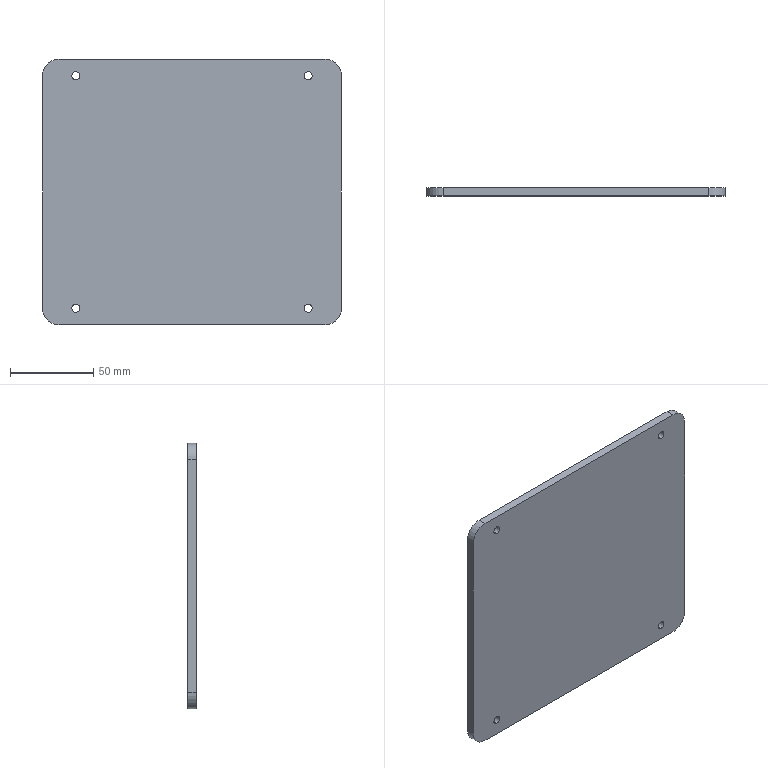Part | SolidWorks | features 3DProfileFeature 1, Extrusion 1, Fillet 1, HoleWzd 1 | 1 solid | 18 faces | box 180 x 5 x 160 mm | volume 143209 mm3 | cylinder 12 | plane 6 | commonest cylinder face diameters 4.8 x8 20 x4
STEP:
#1=CARTESIAN_POINT('',(-70.,-2.5,-72.4));
#2=VERTEX_POINT('',#1);
#3=CARTESIAN_POINT('',(-70.,-2.5,-67.6));
#4=VERTEX_POINT('',#3);
#5=CARTESIAN_POINT('',(-70.,-2.5,-70.));
#6=DIRECTION('',(0.,1.,0.));
#7=DIRECTION('',(0.,0.,1.));
#8=AXIS2_PLACEMENT_3D('',#5,#6,#7);
#9=CIRCLE('',#8,2.4);
#10=EDGE_CURVE('',#2,#4,#9,.T.);
#11=ORIENTED_EDGE('',*,*,#10,.F.);
#12=CARTESIAN_POINT('',(-70.,2.5,-72.4));
#13=VERTEX_POINT('',#12);
#14=CARTESIAN_POINT('',(-70.,2.5,-72.4));
#15=DIRECTION('',(0.,1.,0.));
#16=VECTOR('',#15,1000.);
#17=LINE('',#14,#16);
#18=EDGE_CURVE('',#2,#13,#17,.T.);
#19=ORIENTED_EDGE('',*,*,#18,.T.);
#20=CARTESIAN_POINT('',(-70.,2.5,-67.6));
#21=VERTEX_POINT('',#20);
#22=CARTESIAN_POINT('',(-70.,2.5,-70.));
#23=DIRECTION('',(0.,1.,0.));
#24=DIRECTION('',(0.,0.,1.));
#25=AXIS2_PLACEMENT_3D('',#22,#23,#24);
#26=CIRCLE('',#25,2.4);
#27=EDGE_CURVE('',#13,#21,#26,.T.);
#28=ORIENTED_EDGE('',*,*,#27,.T.);
#29=CARTESIAN_POINT('',(-70.,2.5,-67.6));
#30=DIRECTION('',(0.,1.,0.));
#31=VECTOR('',#30,1000.);
#32=LINE('',#29,#31);
#33=EDGE_CURVE('',#4,#21,#32,.T.);
#34=ORIENTED_EDGE('',*,*,#33,.F.);
#35=EDGE_LOOP('',(#11,#19,#28,#34));
#36=FACE_OUTER_BOUND('',#35,.T.);
#37=CARTESIAN_POINT('',(-70.,2.5,-70.));
#38=DIRECTION('',(0.,1.,0.));
#39=DIRECTION('',(0.,0.,1.));
#40=AXIS2_PLACEMENT_3D('',#37,#38,#39);
#41=CYLINDRICAL_SURFACE('',#40,2.4);
#42=ADVANCED_FACE('',(#36),#41,.F.);
#43=CARTESIAN_POINT('',(70.,-2.5,-72.4));
#44=VERTEX_POINT('',#43);
#45=CARTESIAN_POINT('',(70.,-2.5,-67.6));
#46=VERTEX_POINT('',#45);
#47=CARTESIAN_POINT('',(70.,-2.5,-70.));
#48=DIRECTION('',(0.,1.,0.));
#49=DIRECTION('',(0.,0.,1.));
#50=AXIS2_PLACEMENT_3D('',#47,#48,#49);
#51=CIRCLE('',#50,2.4);
#52=EDGE_CURVE('',#44,#46,#51,.T.);
#53=ORIENTED_EDGE('',*,*,#52,.F.);
#54=CARTESIAN_POINT('',(70.,2.5,-72.4));
#55=VERTEX_POINT('',#54);
#56=CARTESIAN_POINT('',(70.,2.5,-72.4));
#57=DIRECTION('',(0.,1.,0.));
#58=VECTOR('',#57,1000.);
#59=LINE('',#56,#58);
#60=EDGE_CURVE('',#44,#55,#59,.T.);
#61=ORIENTED_EDGE('',*,*,#60,.T.);
#62=CARTESIAN_POINT('',(70.,2.5,-67.6));
#63=VERTEX_POINT('',#62);
#64=CARTESIAN_POINT('',(70.,2.5,-70.));
#65=DIRECTION('',(0.,1.,0.));
#66=DIRECTION('',(0.,0.,1.));
#67=AXIS2_PLACEMENT_3D('',#64,#65,#66);
#68=CIRCLE('',#67,2.4);
#69=EDGE_CURVE('',#55,#63,#68,.T.);
#70=ORIENTED_EDGE('',*,*,#69,.T.);
#71=CARTESIAN_POINT('',(70.,2.5,-67.6));
#72=DIRECTION('',(0.,1.,0.));
#73=VECTOR('',#72,1000.);
#74=LINE('',#71,#73);
#75=EDGE_CURVE('',#46,#63,#74,.T.);
#76=ORIENTED_EDGE('',*,*,#75,.F.);
#77=EDGE_LOOP('',(#53,#61,#70,#76));
#78=FACE_OUTER_BOUND('',#77,.T.);
#79=CARTESIAN_POINT('',(70.,2.5,-70.));
#80=DIRECTION('',(0.,1.,0.));
#81=DIRECTION('',(0.,0.,1.));
#82=AXIS2_PLACEMENT_3D('',#79,#80,#81);
#83=CYLINDRICAL_SURFACE('',#82,2.4);
#84=ADVANCED_FACE('',(#78),#83,.F.);
#85=CARTESIAN_POINT('',(70.,-2.5,67.6));
#86=VERTEX_POINT('',#85);
#87=CARTESIAN_POINT('',(70.,-2.5,72.4));
#88=VERTEX_POINT('',#87);
#89=CARTESIAN_POINT('',(70.,-2.5,70.));
#90=DIRECTION('',(0.,1.,0.));
#91=DIRECTION('',(0.,0.,1.));
#92=AXIS2_PLACEMENT_3D('',#89,#90,#91);
#93=CIRCLE('',#92,2.4);
#94=EDGE_CURVE('',#86,#88,#93,.T.);
#95=ORIENTED_EDGE('',*,*,#94,.F.);
#96=CARTESIAN_POINT('',(70.,2.5,67.6));
#97=VERTEX_POINT('',#96);
#98=CARTESIAN_POINT('',(70.,2.5,67.6));
#99=DIRECTION('',(0.,1.,0.));
#100=VECTOR('',#99,1000.);
#101=LINE('',#98,#100);
#102=EDGE_CURVE('',#86,#97,#101,.T.);
#103=ORIENTED_EDGE('',*,*,#102,.T.);
#104=CARTESIAN_POINT('',(70.,2.5,72.4));
#105=VERTEX_POINT('',#104);
#106=CARTESIAN_POINT('',(70.,2.5,70.));
#107=DIRECTION('',(0.,1.,0.));
#108=DIRECTION('',(0.,0.,1.));
#109=AXIS2_PLACEMENT_3D('',#106,#107,#108);
#110=CIRCLE('',#109,2.4);
#111=EDGE_CURVE('',#97,#105,#110,.T.);
#112=ORIENTED_EDGE('',*,*,#111,.T.);
#113=CARTESIAN_POINT('',(70.,2.5,72.4));
#114=DIRECTION('',(0.,1.,0.));
#115=VECTOR('',#114,1000.);
#116=LINE('',#113,#115);
#117=EDGE_CURVE('',#88,#105,#116,.T.);
#118=ORIENTED_EDGE('',*,*,#117,.F.);
#119=EDGE_LOOP('',(#95,#103,#112,#118));
#120=FACE_OUTER_BOUND('',#119,.T.);
#121=CARTESIAN_POINT('',(70.,2.5,70.));
#122=DIRECTION('',(0.,1.,0.));
#123=DIRECTION('',(0.,0.,1.));
#124=AXIS2_PLACEMENT_3D('',#121,#122,#123);
#125=CYLINDRICAL_SURFACE('',#124,2.4);
#126=ADVANCED_FACE('',(#120),#125,.F.);
#127=CARTESIAN_POINT('',(-70.,-2.5,67.6));
#128=VERTEX_POINT('',#127);
#129=CARTESIAN_POINT('',(-70.,-2.5,72.4));
#130=VERTEX_POINT('',#129);
#131=CARTESIAN_POINT('',(-70.,-2.5,70.));
#132=DIRECTION('',(0.,1.,0.));
#133=DIRECTION('',(0.,0.,1.));
#134=AXIS2_PLACEMENT_3D('',#131,#132,#133);
#135=CIRCLE('',#134,2.4);
#136=EDGE_CURVE('',#128,#130,#135,.T.);
#137=ORIENTED_EDGE('',*,*,#136,.F.);
#138=CARTESIAN_POINT('',(-70.,2.5,67.6));
#139=VERTEX_POINT('',#138);
#140=CARTESIAN_POINT('',(-70.,2.5,67.6));
#141=DIRECTION('',(0.,1.,0.));
#142=VECTOR('',#141,1000.);
#143=LINE('',#140,#142);
#144=EDGE_CURVE('',#128,#139,#143,.T.);
#145=ORIENTED_EDGE('',*,*,#144,.T.);
#146=CARTESIAN_POINT('',(-70.,2.5,72.4));
#147=VERTEX_POINT('',#146);
#148=CARTESIAN_POINT('',(-70.,2.5,70.));
#149=DIRECTION('',(0.,1.,0.));
#150=DIRECTION('',(0.,0.,1.));
#151=AXIS2_PLACEMENT_3D('',#148,#149,#150);
#152=CIRCLE('',#151,2.4);
#153=EDGE_CURVE('',#139,#147,#152,.T.);
#154=ORIENTED_EDGE('',*,*,#153,.T.);
#155=CARTESIAN_POINT('',(-70.,2.5,72.4));
#156=DIRECTION('',(0.,1.,0.));
#157=VECTOR('',#156,1000.);
#158=LINE('',#155,#157);
#159=EDGE_CURVE('',#130,#147,#158,.T.);
#160=ORIENTED_EDGE('',*,*,#159,.F.);
#161=EDGE_LOOP('',(#137,#145,#154,#160));
#162=FACE_OUTER_BOUND('',#161,.T.);
#163=CARTESIAN_POINT('',(-70.,2.5,70.));
#164=DIRECTION('',(0.,1.,0.));
#165=DIRECTION('',(0.,0.,1.));
#166=AXIS2_PLACEMENT_3D('',#163,#164,#165);
#167=CYLINDRICAL_SURFACE('',#166,2.4);
#168=ADVANCED_FACE('',(#162),#167,.F.);
#169=CARTESIAN_POINT('',(90.,2.5,70.));
#170=VERTEX_POINT('',#169);
#171=CARTESIAN_POINT('',(90.,2.5,-70.));
#172=VERTEX_POINT('',#171);
#173=CARTESIAN_POINT('',(90.,2.5,-80.));
#174=DIRECTION('',(0.,0.,-1.));
#175=VECTOR('',#174,1000.);
#176=LINE('',#173,#175);
#177=EDGE_CURVE('',#170,#172,#176,.T.);
#178=ORIENTED_EDGE('',*,*,#177,.F.);
#179=CARTESIAN_POINT('',(90.,-2.5,70.));
#180=VERTEX_POINT('',#179);
#181=CARTESIAN_POINT('',(90.,2.5,70.));
#182=DIRECTION('',(0.,-1.,0.));
#183=VECTOR('',#182,1000.);
#184=LINE('',#181,#183);
#185=EDGE_CURVE('',#170,#180,#184,.T.);
#186=ORIENTED_EDGE('',*,*,#185,.T.);
#187=CARTESIAN_POINT('',(90.,-2.5,-70.));
#188=VERTEX_POINT('',#187);
#189=CARTESIAN_POINT('',(90.,-2.5,-80.));
#190=DIRECTION('',(0.,0.,-1.));
#191=VECTOR('',#190,1000.);
#192=LINE('',#189,#191);
#193=EDGE_CURVE('',#180,#188,#192,.T.);
#194=ORIENTED_EDGE('',*,*,#193,.T.);
#195=CARTESIAN_POINT('',(90.,2.5,-70.));
#196=DIRECTION('',(0.,1.,0.));
#197=VECTOR('',#196,1000.);
#198=LINE('',#195,#197);
#199=EDGE_CURVE('',#188,#172,#198,.T.);
#200=ORIENTED_EDGE('',*,*,#199,.T.);
#201=EDGE_LOOP('',(#178,#186,#194,#200));
#202=FACE_OUTER_BOUND('',#201,.T.);
#203=CARTESIAN_POINT('',(90.,2.5,-80.));
#204=DIRECTION('',(-1.,0.,0.));
#205=DIRECTION('',(0.,0.,1.));
#206=AXIS2_PLACEMENT_3D('',#203,#204,#205);
#207=PLANE('',#206);
#208=ADVANCED_FACE('',(#202),#207,.F.);
#209=CARTESIAN_POINT('',(80.,2.5,-80.));
#210=VERTEX_POINT('',#209);
#211=CARTESIAN_POINT('',(-80.,2.5,-80.));
#212=VERTEX_POINT('',#211);
#213=CARTESIAN_POINT('',(-90.,2.5,-80.));
#214=DIRECTION('',(-1.,0.,0.));
#215=VECTOR('',#214,1000.);
#216=LINE('',#213,#215);
#217=EDGE_CURVE('',#210,#212,#216,.T.);
#218=ORIENTED_EDGE('',*,*,#217,.F.);
#219=CARTESIAN_POINT('',(80.,-2.5,-80.));
#220=VERTEX_POINT('',#219);
#221=CARTESIAN_POINT('',(80.,2.5,-80.));
#222=DIRECTION('',(0.,-1.,0.));
#223=VECTOR('',#222,1000.);
#224=LINE('',#221,#223);
#225=EDGE_CURVE('',#210,#220,#224,.T.);
#226=ORIENTED_EDGE('',*,*,#225,.T.);
#227=CARTESIAN_POINT('',(-80.,-2.5,-80.));
#228=VERTEX_POINT('',#227);
#229=CARTESIAN_POINT('',(-90.,-2.5,-80.));
#230=DIRECTION('',(-1.,0.,0.));
#231=VECTOR('',#230,1000.);
#232=LINE('',#229,#231);
#233=EDGE_CURVE('',#220,#228,#232,.T.);
#234=ORIENTED_EDGE('',*,*,#233,.T.);
#235=CARTESIAN_POINT('',(-80.,2.5,-80.));
#236=DIRECTION('',(0.,1.,0.));
#237=VECTOR('',#236,1000.);
#238=LINE('',#235,#237);
#239=EDGE_CURVE('',#228,#212,#238,.T.);
#240=ORIENTED_EDGE('',*,*,#239,.T.);
#241=EDGE_LOOP('',(#218,#226,#234,#240));
#242=FACE_OUTER_BOUND('',#241,.T.);
#243=CARTESIAN_POINT('',(-90.,2.5,-80.));
#244=DIRECTION('',(0.,0.,1.));
#245=DIRECTION('',(1.,0.,0.));
#246=AXIS2_PLACEMENT_3D('',#243,#244,#245);
#247=PLANE('',#246);
#248=ADVANCED_FACE('',(#242),#247,.F.);
#249=CARTESIAN_POINT('',(-90.,-2.5,-70.));
#250=VERTEX_POINT('',#249);
#251=CARTESIAN_POINT('',(-90.,-2.5,70.));
#252=VERTEX_POINT('',#251);
#253=CARTESIAN_POINT('',(-90.,-2.5,-80.));
#254=DIRECTION('',(0.,0.,1.));
#255=VECTOR('',#254,1000.);
#256=LINE('',#253,#255);
#257=EDGE_CURVE('',#250,#252,#256,.T.);
#258=ORIENTED_EDGE('',*,*,#257,.T.);
#259=CARTESIAN_POINT('',(-90.,2.5,70.));
#260=VERTEX_POINT('',#259);
#261=CARTESIAN_POINT('',(-90.,2.5,70.));
#262=DIRECTION('',(0.,1.,0.));
#263=VECTOR('',#262,1000.);
#264=LINE('',#261,#263);
#265=EDGE_CURVE('',#252,#260,#264,.T.);
#266=ORIENTED_EDGE('',*,*,#265,.T.);
#267=CARTESIAN_POINT('',(-90.,2.5,-70.));
#268=VERTEX_POINT('',#267);
#269=CARTESIAN_POINT('',(-90.,2.5,-80.));
#270=DIRECTION('',(0.,0.,1.));
#271=VECTOR('',#270,1000.);
#272=LINE('',#269,#271);
#273=EDGE_CURVE('',#268,#260,#272,.T.);
#274=ORIENTED_EDGE('',*,*,#273,.F.);
#275=CARTESIAN_POINT('',(-90.,2.5,-70.));
#276=DIRECTION('',(0.,-1.,0.));
#277=VECTOR('',#276,1000.);
#278=LINE('',#275,#277);
#279=EDGE_CURVE('',#268,#250,#278,.T.);
#280=ORIENTED_EDGE('',*,*,#279,.T.);
#281=EDGE_LOOP('',(#258,#266,#274,#280));
#282=FACE_OUTER_BOUND('',#281,.T.);
#283=CARTESIAN_POINT('',(-90.,2.5,-80.));
#284=DIRECTION('',(1.,0.,0.));
#285=DIRECTION('',(0.,0.,-1.));
#286=AXIS2_PLACEMENT_3D('',#283,#284,#285);
#287=PLANE('',#286);
#288=ADVANCED_FACE('',(#282),#287,.F.);
#289=CARTESIAN_POINT('',(-80.,-2.5,80.));
#290=VERTEX_POINT('',#289);
#291=CARTESIAN_POINT('',(80.,-2.5,80.));
#292=VERTEX_POINT('',#291);
#293=CARTESIAN_POINT('',(-90.,-2.5,80.));
#294=DIRECTION('',(1.,0.,0.));
#295=VECTOR('',#294,1000.);
#296=LINE('',#293,#295);
#297=EDGE_CURVE('',#290,#292,#296,.T.);
#298=ORIENTED_EDGE('',*,*,#297,.T.);
#299=CARTESIAN_POINT('',(80.,2.5,80.));
#300=VERTEX_POINT('',#299);
#301=CARTESIAN_POINT('',(80.,2.5,80.));
#302=DIRECTION('',(0.,1.,0.));
#303=VECTOR('',#302,1000.);
#304=LINE('',#301,#303);
#305=EDGE_CURVE('',#292,#300,#304,.T.);
#306=ORIENTED_EDGE('',*,*,#305,.T.);
#307=CARTESIAN_POINT('',(-80.,2.5,80.));
#308=VERTEX_POINT('',#307);
#309=CARTESIAN_POINT('',(-90.,2.5,80.));
#310=DIRECTION('',(1.,0.,0.));
#311=VECTOR('',#310,1000.);
#312=LINE('',#309,#311);
#313=EDGE_CURVE('',#308,#300,#312,.T.);
#314=ORIENTED_EDGE('',*,*,#313,.F.);
#315=CARTESIAN_POINT('',(-80.,2.5,80.));
#316=DIRECTION('',(0.,-1.,0.));
#317=VECTOR('',#316,1000.);
#318=LINE('',#315,#317);
#319=EDGE_CURVE('',#308,#290,#318,.T.);
#320=ORIENTED_EDGE('',*,*,#319,.T.);
#321=EDGE_LOOP('',(#298,#306,#314,#320));
#322=FACE_OUTER_BOUND('',#321,.T.);
#323=CARTESIAN_POINT('',(-90.,2.5,80.));
#324=DIRECTION('',(0.,0.,-1.));
#325=DIRECTION('',(-1.,0.,0.));
#326=AXIS2_PLACEMENT_3D('',#323,#324,#325);
#327=PLANE('',#326);
#328=ADVANCED_FACE('',(#322),#327,.F.);
#329=CARTESIAN_POINT('',(-70.,2.5,-70.));
#330=DIRECTION('',(0.,1.,0.));
#331=DIRECTION('',(0.,0.,1.));
#332=AXIS2_PLACEMENT_3D('',#329,#330,#331);
#333=CIRCLE('',#332,2.4);
#334=EDGE_CURVE('',#21,#13,#333,.T.);
#335=ORIENTED_EDGE('',*,*,#334,.F.);
#336=ORIENTED_EDGE('',*,*,#27,.F.);
#337=EDGE_LOOP('',(#335,#336));
#338=FACE_BOUND('',#337,.T.);
#339=CARTESIAN_POINT('',(70.,2.5,-70.));
#340=DIRECTION('',(0.,1.,0.));
#341=DIRECTION('',(0.,0.,1.));
#342=AXIS2_PLACEMENT_3D('',#339,#340,#341);
#343=CIRCLE('',#342,2.4);
#344=EDGE_CURVE('',#63,#55,#343,.T.);
#345=ORIENTED_EDGE('',*,*,#344,.F.);
#346=ORIENTED_EDGE('',*,*,#69,.F.);
#347=EDGE_LOOP('',(#345,#346));
#348=FACE_BOUND('',#347,.T.);
#349=CARTESIAN_POINT('',(70.,2.5,70.));
#350=DIRECTION('',(0.,1.,0.));
#351=DIRECTION('',(0.,0.,1.));
#352=AXIS2_PLACEMENT_3D('',#349,#350,#351);
#353=CIRCLE('',#352,2.4);
#354=EDGE_CURVE('',#105,#97,#353,.T.);
#355=ORIENTED_EDGE('',*,*,#354,.F.);
#356=ORIENTED_EDGE('',*,*,#111,.F.);
#357=EDGE_LOOP('',(#355,#356));
#358=FACE_BOUND('',#357,.T.);
#359=CARTESIAN_POINT('',(-70.,2.5,70.));
#360=DIRECTION('',(0.,1.,0.));
#361=DIRECTION('',(0.,0.,1.));
#362=AXIS2_PLACEMENT_3D('',#359,#360,#361);
#363=CIRCLE('',#362,2.4);
#364=EDGE_CURVE('',#147,#139,#363,.T.);
#365=ORIENTED_EDGE('',*,*,#364,.F.);
#366=ORIENTED_EDGE('',*,*,#153,.F.);
#367=EDGE_LOOP('',(#365,#366));
#368=FACE_BOUND('',#367,.T.);
#369=ORIENTED_EDGE('',*,*,#313,.T.);
#370=CARTESIAN_POINT('',(80.,2.5,70.));
#371=DIRECTION('',(0.,1.,0.));
#372=DIRECTION('',(0.,0.,1.));
#373=AXIS2_PLACEMENT_3D('',#370,#371,#372);
#374=CIRCLE('',#373,10.);
#375=EDGE_CURVE('',#300,#170,#374,.T.);
#376=ORIENTED_EDGE('',*,*,#375,.T.);
#377=ORIENTED_EDGE('',*,*,#177,.T.);
#378=CARTESIAN_POINT('',(80.,2.5,-70.));
#379=DIRECTION('',(0.,1.,0.));
#380=DIRECTION('',(0.,0.,1.));
#381=AXIS2_PLACEMENT_3D('',#378,#379,#380);
#382=CIRCLE('',#381,10.);
#383=EDGE_CURVE('',#172,#210,#382,.T.);
#384=ORIENTED_EDGE('',*,*,#383,.T.);
#385=ORIENTED_EDGE('',*,*,#217,.T.);
#386=CARTESIAN_POINT('',(-80.,2.5,-70.));
#387=DIRECTION('',(0.,1.,0.));
#388=DIRECTION('',(0.,0.,1.));
#389=AXIS2_PLACEMENT_3D('',#386,#387,#388);
#390=CIRCLE('',#389,10.);
#391=EDGE_CURVE('',#212,#268,#390,.T.);
#392=ORIENTED_EDGE('',*,*,#391,.T.);
#393=ORIENTED_EDGE('',*,*,#273,.T.);
#394=CARTESIAN_POINT('',(-80.,2.5,70.));
#395=DIRECTION('',(0.,1.,0.));
#396=DIRECTION('',(0.,0.,1.));
#397=AXIS2_PLACEMENT_3D('',#394,#395,#396);
#398=CIRCLE('',#397,10.);
#399=EDGE_CURVE('',#260,#308,#398,.T.);
#400=ORIENTED_EDGE('',*,*,#399,.T.);
#401=EDGE_LOOP('',(#369,#376,#377,#384,#385,#392,#393,#400));
#402=FACE_OUTER_BOUND('',#401,.T.);
#403=CARTESIAN_POINT('',(0.,2.5,0.));
#404=DIRECTION('',(0.,1.,0.));
#405=DIRECTION('',(0.,0.,1.));
#406=AXIS2_PLACEMENT_3D('',#403,#404,#405);
#407=PLANE('',#406);
#408=ADVANCED_FACE('',(#338,#348,#358,#368,#402),#407,.T.);
#409=CARTESIAN_POINT('',(-70.,-2.5,-70.));
#410=DIRECTION('',(0.,1.,0.));
#411=DIRECTION('',(0.,0.,1.));
#412=AXIS2_PLACEMENT_3D('',#409,#410,#411);
#413=CIRCLE('',#412,2.4);
#414=EDGE_CURVE('',#4,#2,#413,.T.);
#415=ORIENTED_EDGE('',*,*,#414,.T.);
#416=ORIENTED_EDGE('',*,*,#10,.T.);
#417=EDGE_LOOP('',(#415,#416));
#418=FACE_BOUND('',#417,.T.);
#419=CARTESIAN_POINT('',(70.,-2.5,-70.));
#420=DIRECTION('',(0.,1.,0.));
#421=DIRECTION('',(0.,0.,1.));
#422=AXIS2_PLACEMENT_3D('',#419,#420,#421);
#423=CIRCLE('',#422,2.4);
#424=EDGE_CURVE('',#46,#44,#423,.T.);
#425=ORIENTED_EDGE('',*,*,#424,.T.);
#426=ORIENTED_EDGE('',*,*,#52,.T.);
#427=EDGE_LOOP('',(#425,#426));
#428=FACE_BOUND('',#427,.T.);
#429=CARTESIAN_POINT('',(70.,-2.5,70.));
#430=DIRECTION('',(0.,1.,0.));
#431=DIRECTION('',(0.,0.,1.));
#432=AXIS2_PLACEMENT_3D('',#429,#430,#431);
#433=CIRCLE('',#432,2.4);
#434=EDGE_CURVE('',#88,#86,#433,.T.);
#435=ORIENTED_EDGE('',*,*,#434,.T.);
#436=ORIENTED_EDGE('',*,*,#94,.T.);
#437=EDGE_LOOP('',(#435,#436));
#438=FACE_BOUND('',#437,.T.);
#439=CARTESIAN_POINT('',(-70.,-2.5,70.));
#440=DIRECTION('',(0.,1.,0.));
#441=DIRECTION('',(0.,0.,1.));
#442=AXIS2_PLACEMENT_3D('',#439,#440,#441);
#443=CIRCLE('',#442,2.4);
#444=EDGE_CURVE('',#130,#128,#443,.T.);
#445=ORIENTED_EDGE('',*,*,#444,.T.);
#446=ORIENTED_EDGE('',*,*,#136,.T.);
#447=EDGE_LOOP('',(#445,#446));
#448=FACE_BOUND('',#447,.T.);
#449=ORIENTED_EDGE('',*,*,#193,.F.);
#450=CARTESIAN_POINT('',(80.,-2.5,70.));
#451=DIRECTION('',(0.,-1.,0.));
#452=DIRECTION('',(0.,0.,1.));
#453=AXIS2_PLACEMENT_3D('',#450,#451,#452);
#454=CIRCLE('',#453,10.);
#455=EDGE_CURVE('',#180,#292,#454,.T.);
#456=ORIENTED_EDGE('',*,*,#455,.T.);
#457=ORIENTED_EDGE('',*,*,#297,.F.);
#458=CARTESIAN_POINT('',(-80.,-2.5,70.));
#459=DIRECTION('',(0.,-1.,0.));
#460=DIRECTION('',(0.,0.,1.));
#461=AXIS2_PLACEMENT_3D('',#458,#459,#460);
#462=CIRCLE('',#461,10.);
#463=EDGE_CURVE('',#290,#252,#462,.T.);
#464=ORIENTED_EDGE('',*,*,#463,.T.);
#465=ORIENTED_EDGE('',*,*,#257,.F.);
#466=CARTESIAN_POINT('',(-80.,-2.5,-70.));
#467=DIRECTION('',(0.,-1.,0.));
#468=DIRECTION('',(0.,0.,1.));
#469=AXIS2_PLACEMENT_3D('',#466,#467,#468);
#470=CIRCLE('',#469,10.);
#471=EDGE_CURVE('',#250,#228,#470,.T.);
#472=ORIENTED_EDGE('',*,*,#471,.T.);
#473=ORIENTED_EDGE('',*,*,#233,.F.);
#474=CARTESIAN_POINT('',(80.,-2.5,-70.));
#475=DIRECTION('',(0.,-1.,0.));
#476=DIRECTION('',(0.,0.,1.));
#477=AXIS2_PLACEMENT_3D('',#474,#475,#476);
#478=CIRCLE('',#477,10.);
#479=EDGE_CURVE('',#220,#188,#478,.T.);
#480=ORIENTED_EDGE('',*,*,#479,.T.);
#481=EDGE_LOOP('',(#449,#456,#457,#464,#465,#472,#473,#480));
#482=FACE_OUTER_BOUND('',#481,.T.);
#483=CARTESIAN_POINT('',(0.,-2.5,0.));
#484=DIRECTION('',(0.,1.,0.));
#485=DIRECTION('',(0.,0.,1.));
#486=AXIS2_PLACEMENT_3D('',#483,#484,#485);
#487=PLANE('',#486);
#488=ADVANCED_FACE('',(#418,#428,#438,#448,#482),#487,.F.);
#489=ORIENTED_EDGE('',*,*,#144,.F.);
#490=ORIENTED_EDGE('',*,*,#444,.F.);
#491=ORIENTED_EDGE('',*,*,#159,.T.);
#492=ORIENTED_EDGE('',*,*,#364,.T.);
#493=EDGE_LOOP('',(#489,#490,#491,#492));
#494=FACE_OUTER_BOUND('',#493,.T.);
#495=CARTESIAN_POINT('',(-70.,2.5,70.));
#496=DIRECTION('',(0.,1.,0.));
#497=DIRECTION('',(0.,0.,1.));
#498=AXIS2_PLACEMENT_3D('',#495,#496,#497);
#499=CYLINDRICAL_SURFACE('',#498,2.4);
#500=ADVANCED_FACE('',(#494),#499,.F.);
#501=ORIENTED_EDGE('',*,*,#102,.F.);
#502=ORIENTED_EDGE('',*,*,#434,.F.);
#503=ORIENTED_EDGE('',*,*,#117,.T.);
#504=ORIENTED_EDGE('',*,*,#354,.T.);
#505=EDGE_LOOP('',(#501,#502,#503,#504));
#506=FACE_OUTER_BOUND('',#505,.T.);
#507=CARTESIAN_POINT('',(70.,2.5,70.));
#508=DIRECTION('',(0.,1.,0.));
#509=DIRECTION('',(0.,0.,1.));
#510=AXIS2_PLACEMENT_3D('',#507,#508,#509);
#511=CYLINDRICAL_SURFACE('',#510,2.4);
#512=ADVANCED_FACE('',(#506),#511,.F.);
#513=ORIENTED_EDGE('',*,*,#60,.F.);
#514=ORIENTED_EDGE('',*,*,#424,.F.);
#515=ORIENTED_EDGE('',*,*,#75,.T.);
#516=ORIENTED_EDGE('',*,*,#344,.T.);
#517=EDGE_LOOP('',(#513,#514,#515,#516));
#518=FACE_OUTER_BOUND('',#517,.T.);
#519=CARTESIAN_POINT('',(70.,2.5,-70.));
#520=DIRECTION('',(0.,1.,0.));
#521=DIRECTION('',(0.,0.,1.));
#522=AXIS2_PLACEMENT_3D('',#519,#520,#521);
#523=CYLINDRICAL_SURFACE('',#522,2.4);
#524=ADVANCED_FACE('',(#518),#523,.F.);
#525=ORIENTED_EDGE('',*,*,#18,.F.);
#526=ORIENTED_EDGE('',*,*,#414,.F.);
#527=ORIENTED_EDGE('',*,*,#33,.T.);
#528=ORIENTED_EDGE('',*,*,#334,.T.);
#529=EDGE_LOOP('',(#525,#526,#527,#528));
#530=FACE_OUTER_BOUND('',#529,.T.);
#531=CARTESIAN_POINT('',(-70.,2.5,-70.));
#532=DIRECTION('',(0.,1.,0.));
#533=DIRECTION('',(0.,0.,1.));
#534=AXIS2_PLACEMENT_3D('',#531,#532,#533);
#535=CYLINDRICAL_SURFACE('',#534,2.4);
#536=ADVANCED_FACE('',(#530),#535,.F.);
#537=ORIENTED_EDGE('',*,*,#375,.F.);
#538=ORIENTED_EDGE('',*,*,#305,.F.);
#539=ORIENTED_EDGE('',*,*,#455,.F.);
#540=ORIENTED_EDGE('',*,*,#185,.F.);
#541=EDGE_LOOP('',(#537,#538,#539,#540));
#542=FACE_OUTER_BOUND('',#541,.T.);
#543=CARTESIAN_POINT('',(80.,2.5,70.));
#544=DIRECTION('',(0.,-1.,0.));
#545=DIRECTION('',(0.,0.,-1.));
#546=AXIS2_PLACEMENT_3D('',#543,#544,#545);
#547=CYLINDRICAL_SURFACE('',#546,10.);
#548=ADVANCED_FACE('',(#542),#547,.T.);
#549=ORIENTED_EDGE('',*,*,#399,.F.);
#550=ORIENTED_EDGE('',*,*,#265,.F.);
#551=ORIENTED_EDGE('',*,*,#463,.F.);
#552=ORIENTED_EDGE('',*,*,#319,.F.);
#553=EDGE_LOOP('',(#549,#550,#551,#552));
#554=FACE_OUTER_BOUND('',#553,.T.);
#555=CARTESIAN_POINT('',(-80.,2.5,70.));
#556=DIRECTION('',(0.,-1.,0.));
#557=DIRECTION('',(0.,0.,-1.));
#558=AXIS2_PLACEMENT_3D('',#555,#556,#557);
#559=CYLINDRICAL_SURFACE('',#558,10.);
#560=ADVANCED_FACE('',(#554),#559,.T.);
#561=ORIENTED_EDGE('',*,*,#383,.F.);
#562=ORIENTED_EDGE('',*,*,#199,.F.);
#563=ORIENTED_EDGE('',*,*,#479,.F.);
#564=ORIENTED_EDGE('',*,*,#225,.F.);
#565=EDGE_LOOP('',(#561,#562,#563,#564));
#566=FACE_OUTER_BOUND('',#565,.T.);
#567=CARTESIAN_POINT('',(80.,2.5,-70.));
#568=DIRECTION('',(0.,-1.,0.));
#569=DIRECTION('',(0.,0.,-1.));
#570=AXIS2_PLACEMENT_3D('',#567,#568,#569);
#571=CYLINDRICAL_SURFACE('',#570,10.);
#572=ADVANCED_FACE('',(#566),#571,.T.);
#573=ORIENTED_EDGE('',*,*,#391,.F.);
#574=ORIENTED_EDGE('',*,*,#239,.F.);
#575=ORIENTED_EDGE('',*,*,#471,.F.);
#576=ORIENTED_EDGE('',*,*,#279,.F.);
#577=EDGE_LOOP('',(#573,#574,#575,#576));
#578=FACE_OUTER_BOUND('',#577,.T.);
#579=CARTESIAN_POINT('',(-80.,2.5,-70.));
#580=DIRECTION('',(0.,-1.,0.));
#581=DIRECTION('',(0.,0.,-1.));
#582=AXIS2_PLACEMENT_3D('',#579,#580,#581);
#583=CYLINDRICAL_SURFACE('',#582,10.);
#584=ADVANCED_FACE('',(#578),#583,.T.);
#585=CLOSED_SHELL('',(#42,#84,#126,#168,#208,#248,#288,#328,#408,#488,#500,#512,#524,#536,#548,#560,#572,#584));
#586=MANIFOLD_SOLID_BREP('',#585);
#587=CARTESIAN_POINT('',(0.,0.,0.));
#588=DIRECTION('',(0.,0.,1.));
#589=DIRECTION('',(1.,0.,0.));
#590=AXIS2_PLACEMENT_3D('',#587,#588,#589);
#591=(LENGTH_UNIT()NAMED_UNIT(*)SI_UNIT(.MILLI.,.METRE.));
#592=UNCERTAINTY_MEASURE_WITH_UNIT(LENGTH_MEASURE(0.00001),#591,'','');
#593=(NAMED_UNIT(*)PLANE_ANGLE_UNIT()SI_UNIT($,.RADIAN.));
#594=(NAMED_UNIT(*)SI_UNIT($,.STERADIAN.)SOLID_ANGLE_UNIT());
#595=(GEOMETRIC_REPRESENTATION_CONTEXT(3)GLOBAL_UNCERTAINTY_ASSIGNED_CONTEXT((#592))GLOBAL_UNIT_ASSIGNED_CONTEXT((#591,#593,#594))REPRESENTATION_CONTEXT('',''));
#596=ADVANCED_BREP_SHAPE_REPRESENTATION('',(#586,#590),#595);